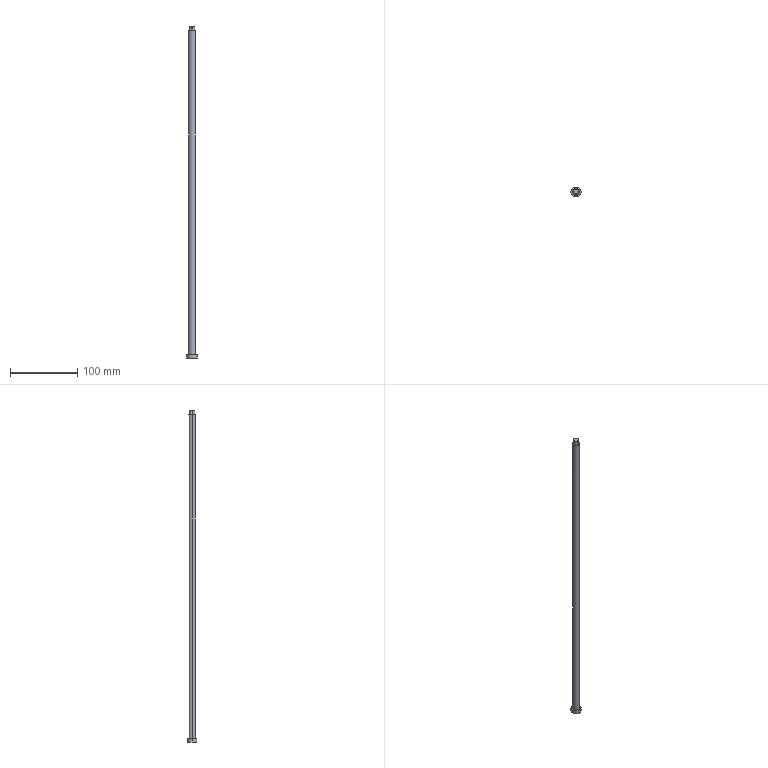Part | SolidWorks | features BaseBody 1 | 1 solid | 14 faces | box 15 x 15 x 495 mm | volume 39144 mm3 | cylinder 8 | plane 4 | cone 2 | commonest cylinder face diameters 2 x2 8 x2 10 x2 15 x2
STEP:
#1=CARTESIAN_POINT('',(-3.75,0.,495.));
#2=VERTEX_POINT('',#1);
#3=CARTESIAN_POINT('',(3.75,0.,495.));
#4=VERTEX_POINT('',#3);
#5=CARTESIAN_POINT('',(0.,0.,495.));
#6=DIRECTION('',(0.,0.,-1.));
#7=DIRECTION('',(-1.,0.,0.));
#8=AXIS2_PLACEMENT_3D('',#5,#6,#7);
#9=CIRCLE('',#8,3.75);
#10=EDGE_CURVE('',#2,#4,#9,.T.);
#11=ORIENTED_EDGE('',*,*,#10,.T.);
#12=CARTESIAN_POINT('',(4.,0.,494.75));
#13=VERTEX_POINT('',#12);
#14=CARTESIAN_POINT('',(3.875,0.,494.875));
#15=DIRECTION('',(0.7071,0.,-0.7071));
#16=VECTOR('',#15,1000.);
#17=LINE('',#14,#16);
#18=EDGE_CURVE('',#4,#13,#17,.T.);
#19=ORIENTED_EDGE('',*,*,#18,.T.);
#20=CARTESIAN_POINT('',(-4.,0.,494.75));
#21=VERTEX_POINT('',#20);
#22=CARTESIAN_POINT('',(0.,0.,494.75));
#23=DIRECTION('',(0.,0.,1.));
#24=DIRECTION('',(-1.,0.,0.));
#25=AXIS2_PLACEMENT_3D('',#22,#23,#24);
#26=CIRCLE('',#25,4.);
#27=EDGE_CURVE('',#13,#21,#26,.T.);
#28=ORIENTED_EDGE('',*,*,#27,.T.);
#29=CARTESIAN_POINT('',(-3.875,0.,494.875));
#30=DIRECTION('',(-0.7071,0.,-0.7071));
#31=VECTOR('',#30,1000.);
#32=LINE('',#29,#31);
#33=EDGE_CURVE('',#2,#21,#32,.T.);
#34=ORIENTED_EDGE('',*,*,#33,.F.);
#35=EDGE_LOOP('',(#11,#19,#28,#34));
#36=FACE_OUTER_BOUND('',#35,.T.);
#37=CARTESIAN_POINT('',(0.,0.,494.875));
#38=DIRECTION('',(0.,0.,-1.));
#39=DIRECTION('',(-1.,0.,0.));
#40=AXIS2_PLACEMENT_3D('',#37,#38,#39);
#41=CONICAL_SURFACE('',#40,3.875,0.7854);
#42=ADVANCED_FACE('',(#36),#41,.T.);
#43=CARTESIAN_POINT('',(1.,-3.873,493.));
#44=VERTEX_POINT('',#43);
#45=CARTESIAN_POINT('',(-1.,-3.873,493.));
#46=VERTEX_POINT('',#45);
#47=CARTESIAN_POINT('',(1.,-3.873,493.));
#48=CARTESIAN_POINT('',(1.,-3.873,493.133));
#49=CARTESIAN_POINT('',(0.9737,-3.88,493.263));
#50=CARTESIAN_POINT('',(0.8732,-3.904,493.505));
#51=CARTESIAN_POINT('',(0.7989,-3.921,493.615));
#52=CARTESIAN_POINT('',(0.6153,-3.953,493.799));
#53=CARTESIAN_POINT('',(0.5042,-3.97,493.873));
#54=CARTESIAN_POINT('',(0.2638,-3.993,493.973));
#55=CARTESIAN_POINT('',(0.1319,-4.,494.));
#56=CARTESIAN_POINT('',(-0.1301,-4.,494.));
#57=CARTESIAN_POINT('',(-0.2614,-3.993,493.974));
#58=CARTESIAN_POINT('',(-0.5042,-3.97,493.874));
#59=CARTESIAN_POINT('',(-0.6141,-3.954,493.8));
#60=CARTESIAN_POINT('',(-0.7995,-3.92,493.615));
#61=CARTESIAN_POINT('',(-0.8731,-3.904,493.505));
#62=CARTESIAN_POINT('',(-0.9735,-3.88,493.263));
#63=CARTESIAN_POINT('',(-1.,-3.873,493.133));
#64=CARTESIAN_POINT('',(-1.,-3.873,493.));
#65=B_SPLINE_CURVE_WITH_KNOTS('',3,(#47,#48,#49,#50,#51,#52,#53,#54,#55,#56,#57,#58,#59,#60,#61,#62,#63,#64),.UNSPECIFIED.,.F.,.F.,(4,2,2,2,2,2,2,2,4),(0.,0.0003922,0.0007845,0.001177,0.001569,0.001961,0.002353,0.002746,0.003138),.UNSPECIFIED.);
#66=EDGE_CURVE('',#44,#46,#65,.T.);
#67=ORIENTED_EDGE('',*,*,#66,.F.);
#68=CARTESIAN_POINT('',(-1.,-3.873,493.));
#69=CARTESIAN_POINT('',(-1.,-3.873,492.867));
#70=CARTESIAN_POINT('',(-0.9737,-3.88,492.737));
#71=CARTESIAN_POINT('',(-0.8732,-3.904,492.495));
#72=CARTESIAN_POINT('',(-0.7989,-3.921,492.385));
#73=CARTESIAN_POINT('',(-0.6153,-3.953,492.201));
#74=CARTESIAN_POINT('',(-0.5042,-3.97,492.127));
#75=CARTESIAN_POINT('',(-0.2638,-3.993,492.027));
#76=CARTESIAN_POINT('',(-0.1319,-4.,492.));
#77=CARTESIAN_POINT('',(0.1301,-4.,492.));
#78=CARTESIAN_POINT('',(0.2614,-3.993,492.026));
#79=CARTESIAN_POINT('',(0.5042,-3.97,492.126));
#80=CARTESIAN_POINT('',(0.6141,-3.954,492.2));
#81=CARTESIAN_POINT('',(0.7995,-3.92,492.385));
#82=CARTESIAN_POINT('',(0.8731,-3.904,492.495));
#83=CARTESIAN_POINT('',(0.9735,-3.88,492.737));
#84=CARTESIAN_POINT('',(1.,-3.873,492.867));
#85=CARTESIAN_POINT('',(1.,-3.873,493.));
#86=B_SPLINE_CURVE_WITH_KNOTS('',3,(#68,#69,#70,#71,#72,#73,#74,#75,#76,#77,#78,#79,#80,#81,#82,#83,#84,#85),.UNSPECIFIED.,.F.,.F.,(4,2,2,2,2,2,2,2,4),(0.003138,0.00353,0.003922,0.004315,0.004707,0.005099,0.005491,0.005884,0.006276),.UNSPECIFIED.);
#87=EDGE_CURVE('',#46,#44,#86,.T.);
#88=ORIENTED_EDGE('',*,*,#87,.F.);
#89=EDGE_LOOP('',(#67,#88));
#90=FACE_BOUND('',#89,.T.);
#91=CARTESIAN_POINT('',(-4.,0.,488.));
#92=VERTEX_POINT('',#91);
#93=CARTESIAN_POINT('',(4.,0.,488.));
#94=VERTEX_POINT('',#93);
#95=CARTESIAN_POINT('',(0.,0.,488.));
#96=DIRECTION('',(0.,0.,1.));
#97=DIRECTION('',(-1.,0.,0.));
#98=AXIS2_PLACEMENT_3D('',#95,#96,#97);
#99=CIRCLE('',#98,4.);
#100=EDGE_CURVE('',#92,#94,#99,.T.);
#101=ORIENTED_EDGE('',*,*,#100,.T.);
#102=CARTESIAN_POINT('',(4.,0.,495.));
#103=DIRECTION('',(0.,0.,1.));
#104=VECTOR('',#103,1000.);
#105=LINE('',#102,#104);
#106=EDGE_CURVE('',#94,#13,#105,.T.);
#107=ORIENTED_EDGE('',*,*,#106,.T.);
#108=CARTESIAN_POINT('',(0.,0.,494.75));
#109=DIRECTION('',(0.,0.,1.));
#110=DIRECTION('',(-1.,0.,0.));
#111=AXIS2_PLACEMENT_3D('',#108,#109,#110);
#112=CIRCLE('',#111,4.);
#113=EDGE_CURVE('',#21,#13,#112,.T.);
#114=ORIENTED_EDGE('',*,*,#113,.F.);
#115=CARTESIAN_POINT('',(-4.,0.,495.));
#116=DIRECTION('',(0.,0.,1.));
#117=VECTOR('',#116,1000.);
#118=LINE('',#115,#117);
#119=EDGE_CURVE('',#92,#21,#118,.T.);
#120=ORIENTED_EDGE('',*,*,#119,.F.);
#121=EDGE_LOOP('',(#101,#107,#114,#120));
#122=FACE_OUTER_BOUND('',#121,.T.);
#123=CARTESIAN_POINT('',(0.,0.,495.));
#124=DIRECTION('',(0.,0.,1.));
#125=DIRECTION('',(-1.,0.,0.));
#126=AXIS2_PLACEMENT_3D('',#123,#124,#125);
#127=CYLINDRICAL_SURFACE('',#126,4.);
#128=ADVANCED_FACE('',(#90,#122),#127,.T.);
#129=CARTESIAN_POINT('',(1.,3.873,493.));
#130=VERTEX_POINT('',#129);
#131=CARTESIAN_POINT('',(-1.,3.873,493.));
#132=VERTEX_POINT('',#131);
#133=CARTESIAN_POINT('',(1.,3.873,493.));
#134=CARTESIAN_POINT('',(1.,3.873,492.867));
#135=CARTESIAN_POINT('',(0.9737,3.88,492.737));
#136=CARTESIAN_POINT('',(0.8732,3.904,492.495));
#137=CARTESIAN_POINT('',(0.7989,3.921,492.385));
#138=CARTESIAN_POINT('',(0.6153,3.953,492.201));
#139=CARTESIAN_POINT('',(0.5042,3.97,492.127));
#140=CARTESIAN_POINT('',(0.2638,3.993,492.027));
#141=CARTESIAN_POINT('',(0.1319,4.,492.));
#142=CARTESIAN_POINT('',(-0.1301,4.,492.));
#143=CARTESIAN_POINT('',(-0.2614,3.993,492.026));
#144=CARTESIAN_POINT('',(-0.5042,3.97,492.126));
#145=CARTESIAN_POINT('',(-0.6141,3.954,492.2));
#146=CARTESIAN_POINT('',(-0.7995,3.92,492.385));
#147=CARTESIAN_POINT('',(-0.8731,3.904,492.495));
#148=CARTESIAN_POINT('',(-0.9735,3.88,492.737));
#149=CARTESIAN_POINT('',(-1.,3.873,492.867));
#150=CARTESIAN_POINT('',(-1.,3.873,493.));
#151=B_SPLINE_CURVE_WITH_KNOTS('',3,(#133,#134,#135,#136,#137,#138,#139,#140,#141,#142,#143,#144,#145,#146,#147,#148,#149,#150),.UNSPECIFIED.,.F.,.F.,(4,2,2,2,2,2,2,2,4),(0.,0.0003922,0.0007845,0.001177,0.001569,0.001961,0.002353,0.002746,0.003138),.UNSPECIFIED.);
#152=EDGE_CURVE('',#130,#132,#151,.T.);
#153=ORIENTED_EDGE('',*,*,#152,.T.);
#154=CARTESIAN_POINT('',(-1.,0.,493.));
#155=DIRECTION('',(0.,-1.,0.));
#156=VECTOR('',#155,1000.);
#157=LINE('',#154,#156);
#158=EDGE_CURVE('',#132,#46,#157,.T.);
#159=ORIENTED_EDGE('',*,*,#158,.T.);
#160=ORIENTED_EDGE('',*,*,#87,.T.);
#161=CARTESIAN_POINT('',(1.,0.,493.));
#162=DIRECTION('',(0.,-1.,0.));
#163=VECTOR('',#162,1000.);
#164=LINE('',#161,#163);
#165=EDGE_CURVE('',#130,#44,#164,.T.);
#166=ORIENTED_EDGE('',*,*,#165,.F.);
#167=EDGE_LOOP('',(#153,#159,#160,#166));
#168=FACE_OUTER_BOUND('',#167,.T.);
#169=CARTESIAN_POINT('',(0.,0.,493.));
#170=DIRECTION('',(0.,-1.,0.));
#171=DIRECTION('',(1.,0.,0.));
#172=AXIS2_PLACEMENT_3D('',#169,#170,#171);
#173=CYLINDRICAL_SURFACE('',#172,1.);
#174=ADVANCED_FACE('',(#168),#173,.F.);
#175=CARTESIAN_POINT('',(-5.,0.,488.));
#176=VERTEX_POINT('',#175);
#177=CARTESIAN_POINT('',(5.,0.,488.));
#178=VERTEX_POINT('',#177);
#179=CARTESIAN_POINT('',(0.,0.,488.));
#180=DIRECTION('',(0.,0.,-1.));
#181=DIRECTION('',(-1.,0.,0.));
#182=AXIS2_PLACEMENT_3D('',#179,#180,#181);
#183=CIRCLE('',#182,5.);
#184=EDGE_CURVE('',#176,#178,#183,.T.);
#185=ORIENTED_EDGE('',*,*,#184,.T.);
#186=CARTESIAN_POINT('',(5.,0.,5.));
#187=VERTEX_POINT('',#186);
#188=CARTESIAN_POINT('',(5.,0.,5.));
#189=DIRECTION('',(0.,0.,-1.));
#190=VECTOR('',#189,1000.);
#191=LINE('',#188,#190);
#192=EDGE_CURVE('',#178,#187,#191,.T.);
#193=ORIENTED_EDGE('',*,*,#192,.T.);
#194=CARTESIAN_POINT('',(-5.,0.,5.));
#195=VERTEX_POINT('',#194);
#196=CARTESIAN_POINT('',(0.,0.,5.));
#197=DIRECTION('',(0.,0.,-1.));
#198=DIRECTION('',(-1.,0.,0.));
#199=AXIS2_PLACEMENT_3D('',#196,#197,#198);
#200=CIRCLE('',#199,5.);
#201=EDGE_CURVE('',#195,#187,#200,.T.);
#202=ORIENTED_EDGE('',*,*,#201,.F.);
#203=CARTESIAN_POINT('',(-5.,0.,5.));
#204=DIRECTION('',(0.,0.,-1.));
#205=VECTOR('',#204,1000.);
#206=LINE('',#203,#205);
#207=EDGE_CURVE('',#176,#195,#206,.T.);
#208=ORIENTED_EDGE('',*,*,#207,.F.);
#209=EDGE_LOOP('',(#185,#193,#202,#208));
#210=FACE_OUTER_BOUND('',#209,.T.);
#211=CARTESIAN_POINT('',(0.,0.,5.));
#212=DIRECTION('',(0.,0.,-1.));
#213=DIRECTION('',(-1.,0.,0.));
#214=AXIS2_PLACEMENT_3D('',#211,#212,#213);
#215=CYLINDRICAL_SURFACE('',#214,5.);
#216=ADVANCED_FACE('',(#210),#215,.T.);
#217=CARTESIAN_POINT('',(7.5,0.,5.));
#218=VERTEX_POINT('',#217);
#219=CARTESIAN_POINT('',(-7.5,0.,5.));
#220=VERTEX_POINT('',#219);
#221=CARTESIAN_POINT('',(0.,0.,5.));
#222=DIRECTION('',(0.,0.,1.));
#223=DIRECTION('',(-1.,0.,0.));
#224=AXIS2_PLACEMENT_3D('',#221,#222,#223);
#225=CIRCLE('',#224,7.5);
#226=EDGE_CURVE('',#218,#220,#225,.T.);
#227=ORIENTED_EDGE('',*,*,#226,.F.);
#228=CARTESIAN_POINT('',(7.5,0.,0.));
#229=VERTEX_POINT('',#228);
#230=CARTESIAN_POINT('',(7.5,0.,0.));
#231=DIRECTION('',(0.,0.,-1.));
#232=VECTOR('',#231,1000.);
#233=LINE('',#230,#232);
#234=EDGE_CURVE('',#218,#229,#233,.T.);
#235=ORIENTED_EDGE('',*,*,#234,.T.);
#236=CARTESIAN_POINT('',(-7.5,0.,0.));
#237=VERTEX_POINT('',#236);
#238=CARTESIAN_POINT('',(0.,0.,0.));
#239=DIRECTION('',(0.,0.,-1.));
#240=DIRECTION('',(-1.,0.,0.));
#241=AXIS2_PLACEMENT_3D('',#238,#239,#240);
#242=CIRCLE('',#241,7.5);
#243=EDGE_CURVE('',#237,#229,#242,.T.);
#244=ORIENTED_EDGE('',*,*,#243,.F.);
#245=CARTESIAN_POINT('',(-7.5,0.,0.));
#246=DIRECTION('',(0.,0.,-1.));
#247=VECTOR('',#246,1000.);
#248=LINE('',#245,#247);
#249=EDGE_CURVE('',#220,#237,#248,.T.);
#250=ORIENTED_EDGE('',*,*,#249,.F.);
#251=EDGE_LOOP('',(#227,#235,#244,#250));
#252=FACE_OUTER_BOUND('',#251,.T.);
#253=CARTESIAN_POINT('',(0.,0.,0.));
#254=DIRECTION('',(0.,0.,-1.));
#255=DIRECTION('',(-1.,0.,0.));
#256=AXIS2_PLACEMENT_3D('',#253,#254,#255);
#257=CYLINDRICAL_SURFACE('',#256,7.5);
#258=ADVANCED_FACE('',(#252),#257,.T.);
#259=ORIENTED_EDGE('',*,*,#10,.F.);
#260=CARTESIAN_POINT('',(0.,0.,495.));
#261=DIRECTION('',(0.,0.,-1.));
#262=DIRECTION('',(-1.,0.,0.));
#263=AXIS2_PLACEMENT_3D('',#260,#261,#262);
#264=CIRCLE('',#263,3.75);
#265=EDGE_CURVE('',#4,#2,#264,.T.);
#266=ORIENTED_EDGE('',*,*,#265,.F.);
#267=EDGE_LOOP('',(#259,#266));
#268=FACE_OUTER_BOUND('',#267,.T.);
#269=CARTESIAN_POINT('',(0.,0.,495.));
#270=DIRECTION('',(0.,0.,1.));
#271=DIRECTION('',(1.,0.,0.));
#272=AXIS2_PLACEMENT_3D('',#269,#270,#271);
#273=PLANE('',#272);
#274=ADVANCED_FACE('',(#268),#273,.T.);
#275=ORIENTED_EDGE('',*,*,#100,.F.);
#276=CARTESIAN_POINT('',(0.,0.,488.));
#277=DIRECTION('',(0.,0.,1.));
#278=DIRECTION('',(-1.,0.,0.));
#279=AXIS2_PLACEMENT_3D('',#276,#277,#278);
#280=CIRCLE('',#279,4.);
#281=EDGE_CURVE('',#94,#92,#280,.T.);
#282=ORIENTED_EDGE('',*,*,#281,.F.);
#283=EDGE_LOOP('',(#275,#282));
#284=FACE_BOUND('',#283,.T.);
#285=ORIENTED_EDGE('',*,*,#184,.F.);
#286=CARTESIAN_POINT('',(0.,0.,488.));
#287=DIRECTION('',(0.,0.,-1.));
#288=DIRECTION('',(-1.,0.,0.));
#289=AXIS2_PLACEMENT_3D('',#286,#287,#288);
#290=CIRCLE('',#289,5.);
#291=EDGE_CURVE('',#178,#176,#290,.T.);
#292=ORIENTED_EDGE('',*,*,#291,.F.);
#293=EDGE_LOOP('',(#285,#292));
#294=FACE_OUTER_BOUND('',#293,.T.);
#295=CARTESIAN_POINT('',(0.,0.,488.));
#296=DIRECTION('',(0.,0.,1.));
#297=DIRECTION('',(1.,0.,0.));
#298=AXIS2_PLACEMENT_3D('',#295,#296,#297);
#299=PLANE('',#298);
#300=ADVANCED_FACE('',(#284,#294),#299,.T.);
#301=ORIENTED_EDGE('',*,*,#243,.T.);
#302=CARTESIAN_POINT('',(0.,0.,0.));
#303=DIRECTION('',(0.,0.,-1.));
#304=DIRECTION('',(-1.,0.,0.));
#305=AXIS2_PLACEMENT_3D('',#302,#303,#304);
#306=CIRCLE('',#305,7.5);
#307=EDGE_CURVE('',#229,#237,#306,.T.);
#308=ORIENTED_EDGE('',*,*,#307,.T.);
#309=EDGE_LOOP('',(#301,#308));
#310=FACE_OUTER_BOUND('',#309,.T.);
#311=CARTESIAN_POINT('',(0.,0.,0.));
#312=DIRECTION('',(0.,0.,1.));
#313=DIRECTION('',(1.,0.,0.));
#314=AXIS2_PLACEMENT_3D('',#311,#312,#313);
#315=PLANE('',#314);
#316=ADVANCED_FACE('',(#310),#315,.F.);
#317=ORIENTED_EDGE('',*,*,#201,.T.);
#318=CARTESIAN_POINT('',(0.,0.,5.));
#319=DIRECTION('',(0.,0.,-1.));
#320=DIRECTION('',(-1.,0.,0.));
#321=AXIS2_PLACEMENT_3D('',#318,#319,#320);
#322=CIRCLE('',#321,5.);
#323=EDGE_CURVE('',#187,#195,#322,.T.);
#324=ORIENTED_EDGE('',*,*,#323,.T.);
#325=EDGE_LOOP('',(#317,#324));
#326=FACE_BOUND('',#325,.T.);
#327=CARTESIAN_POINT('',(0.,0.,5.));
#328=DIRECTION('',(0.,0.,1.));
#329=DIRECTION('',(-1.,0.,0.));
#330=AXIS2_PLACEMENT_3D('',#327,#328,#329);
#331=CIRCLE('',#330,7.5);
#332=EDGE_CURVE('',#220,#218,#331,.T.);
#333=ORIENTED_EDGE('',*,*,#332,.T.);
#334=ORIENTED_EDGE('',*,*,#226,.T.);
#335=EDGE_LOOP('',(#333,#334));
#336=FACE_OUTER_BOUND('',#335,.T.);
#337=CARTESIAN_POINT('',(0.,0.,5.));
#338=DIRECTION('',(0.,0.,1.));
#339=DIRECTION('',(1.,0.,0.));
#340=AXIS2_PLACEMENT_3D('',#337,#338,#339);
#341=PLANE('',#340);
#342=ADVANCED_FACE('',(#326,#336),#341,.T.);
#343=ORIENTED_EDGE('',*,*,#234,.F.);
#344=ORIENTED_EDGE('',*,*,#332,.F.);
#345=ORIENTED_EDGE('',*,*,#249,.T.);
#346=ORIENTED_EDGE('',*,*,#307,.F.);
#347=EDGE_LOOP('',(#343,#344,#345,#346));
#348=FACE_OUTER_BOUND('',#347,.T.);
#349=CARTESIAN_POINT('',(0.,0.,0.));
#350=DIRECTION('',(0.,0.,-1.));
#351=DIRECTION('',(-1.,0.,0.));
#352=AXIS2_PLACEMENT_3D('',#349,#350,#351);
#353=CYLINDRICAL_SURFACE('',#352,7.5);
#354=ADVANCED_FACE('',(#348),#353,.T.);
#355=ORIENTED_EDGE('',*,*,#192,.F.);
#356=ORIENTED_EDGE('',*,*,#291,.T.);
#357=ORIENTED_EDGE('',*,*,#207,.T.);
#358=ORIENTED_EDGE('',*,*,#323,.F.);
#359=EDGE_LOOP('',(#355,#356,#357,#358));
#360=FACE_OUTER_BOUND('',#359,.T.);
#361=CARTESIAN_POINT('',(0.,0.,5.));
#362=DIRECTION('',(0.,0.,-1.));
#363=DIRECTION('',(-1.,0.,0.));
#364=AXIS2_PLACEMENT_3D('',#361,#362,#363);
#365=CYLINDRICAL_SURFACE('',#364,5.);
#366=ADVANCED_FACE('',(#360),#365,.T.);
#367=ORIENTED_EDGE('',*,*,#158,.F.);
#368=CARTESIAN_POINT('',(-1.,3.873,493.));
#369=CARTESIAN_POINT('',(-1.,3.873,493.133));
#370=CARTESIAN_POINT('',(-0.9737,3.88,493.263));
#371=CARTESIAN_POINT('',(-0.8732,3.904,493.505));
#372=CARTESIAN_POINT('',(-0.7989,3.921,493.615));
#373=CARTESIAN_POINT('',(-0.6153,3.953,493.799));
#374=CARTESIAN_POINT('',(-0.5042,3.97,493.873));
#375=CARTESIAN_POINT('',(-0.2638,3.993,493.973));
#376=CARTESIAN_POINT('',(-0.1319,4.,494.));
#377=CARTESIAN_POINT('',(0.1301,4.,494.));
#378=CARTESIAN_POINT('',(0.2614,3.993,493.974));
#379=CARTESIAN_POINT('',(0.5042,3.97,493.874));
#380=CARTESIAN_POINT('',(0.6141,3.954,493.8));
#381=CARTESIAN_POINT('',(0.7995,3.92,493.615));
#382=CARTESIAN_POINT('',(0.8731,3.904,493.505));
#383=CARTESIAN_POINT('',(0.9735,3.88,493.263));
#384=CARTESIAN_POINT('',(1.,3.873,493.133));
#385=CARTESIAN_POINT('',(1.,3.873,493.));
#386=B_SPLINE_CURVE_WITH_KNOTS('',3,(#368,#369,#370,#371,#372,#373,#374,#375,#376,#377,#378,#379,#380,#381,#382,#383,#384,#385),.UNSPECIFIED.,.F.,.F.,(4,2,2,2,2,2,2,2,4),(0.003138,0.00353,0.003922,0.004315,0.004707,0.005099,0.005491,0.005884,0.006276),.UNSPECIFIED.);
#387=EDGE_CURVE('',#132,#130,#386,.T.);
#388=ORIENTED_EDGE('',*,*,#387,.T.);
#389=ORIENTED_EDGE('',*,*,#165,.T.);
#390=ORIENTED_EDGE('',*,*,#66,.T.);
#391=EDGE_LOOP('',(#367,#388,#389,#390));
#392=FACE_OUTER_BOUND('',#391,.T.);
#393=CARTESIAN_POINT('',(0.,0.,493.));
#394=DIRECTION('',(0.,-1.,0.));
#395=DIRECTION('',(1.,0.,0.));
#396=AXIS2_PLACEMENT_3D('',#393,#394,#395);
#397=CYLINDRICAL_SURFACE('',#396,1.);
#398=ADVANCED_FACE('',(#392),#397,.F.);
#399=ORIENTED_EDGE('',*,*,#106,.F.);
#400=ORIENTED_EDGE('',*,*,#281,.T.);
#401=ORIENTED_EDGE('',*,*,#119,.T.);
#402=ORIENTED_EDGE('',*,*,#27,.F.);
#403=EDGE_LOOP('',(#399,#400,#401,#402));
#404=FACE_OUTER_BOUND('',#403,.T.);
#405=ORIENTED_EDGE('',*,*,#152,.F.);
#406=ORIENTED_EDGE('',*,*,#387,.F.);
#407=EDGE_LOOP('',(#405,#406));
#408=FACE_BOUND('',#407,.T.);
#409=CARTESIAN_POINT('',(0.,0.,495.));
#410=DIRECTION('',(0.,0.,1.));
#411=DIRECTION('',(-1.,0.,0.));
#412=AXIS2_PLACEMENT_3D('',#409,#410,#411);
#413=CYLINDRICAL_SURFACE('',#412,4.);
#414=ADVANCED_FACE('',(#404,#408),#413,.T.);
#415=ORIENTED_EDGE('',*,*,#18,.F.);
#416=ORIENTED_EDGE('',*,*,#265,.T.);
#417=ORIENTED_EDGE('',*,*,#33,.T.);
#418=ORIENTED_EDGE('',*,*,#113,.T.);
#419=EDGE_LOOP('',(#415,#416,#417,#418));
#420=FACE_OUTER_BOUND('',#419,.T.);
#421=CARTESIAN_POINT('',(0.,0.,494.875));
#422=DIRECTION('',(0.,0.,-1.));
#423=DIRECTION('',(-1.,0.,0.));
#424=AXIS2_PLACEMENT_3D('',#421,#422,#423);
#425=CONICAL_SURFACE('',#424,3.875,0.7854);
#426=ADVANCED_FACE('',(#420),#425,.T.);
#427=CLOSED_SHELL('',(#42,#128,#174,#216,#258,#274,#300,#316,#342,#354,#366,#398,#414,#426));
#428=MANIFOLD_SOLID_BREP('',#427);
#429=CARTESIAN_POINT('',(0.,0.,0.));
#430=DIRECTION('',(0.,0.,1.));
#431=DIRECTION('',(1.,0.,0.));
#432=AXIS2_PLACEMENT_3D('',#429,#430,#431);
#433=(LENGTH_UNIT()NAMED_UNIT(*)SI_UNIT(.MILLI.,.METRE.));
#434=UNCERTAINTY_MEASURE_WITH_UNIT(LENGTH_MEASURE(0.00001),#433,'','');
#435=(NAMED_UNIT(*)PLANE_ANGLE_UNIT()SI_UNIT($,.RADIAN.));
#436=(NAMED_UNIT(*)SI_UNIT($,.STERADIAN.)SOLID_ANGLE_UNIT());
#437=(GEOMETRIC_REPRESENTATION_CONTEXT(3)GLOBAL_UNCERTAINTY_ASSIGNED_CONTEXT((#434))GLOBAL_UNIT_ASSIGNED_CONTEXT((#433,#435,#436))REPRESENTATION_CONTEXT('',''));
#438=ADVANCED_BREP_SHAPE_REPRESENTATION('',(#428,#432),#437);